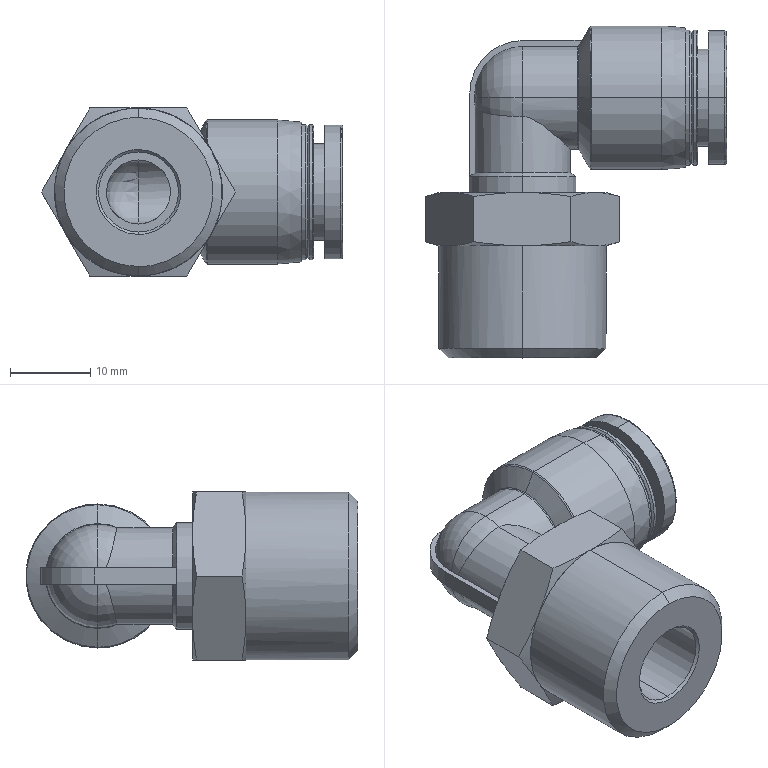Part | SolidWorks | features BaseBody 1 | 1 solid | 94 faces | box 37.624 x 41.5 x 21 mm | volume 10136 mm3 | cylinder 29 | cone 28 | plane 19 | torus 17 | sphere 1 | commonest cylinder face diameters 8 x4 10 x4 16.9 x4 12 x3 12.9 x3 13.4 x3